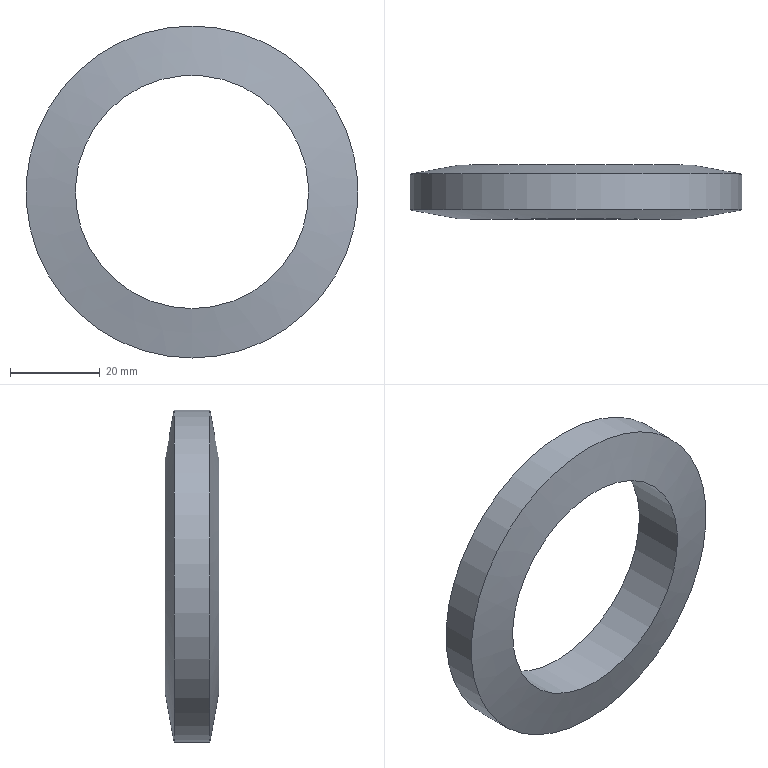Part | NX | features DATUM_CSYS 2, SKETCH 1, SWP104 1 | 1 solid | 4 faces | box 74 x 12 x 74 mm | volume 21518 mm3 | cone 2 | cylinder 2 | commonest cylinder face diameters 52 x1 74 x1
STEP:
#1=CARTESIAN_POINT('',(0.,-6.,-26.));
#2=VERTEX_POINT('',#1);
#3=CARTESIAN_POINT('',(0.,-6.,0.));
#4=DIRECTION('',(0.,-1.,0.));
#5=DIRECTION('',(0.,0.,-1.));
#6=AXIS2_PLACEMENT_3D('',#3,#4,#5);
#7=CIRCLE('',#6,26.);
#8=EDGE_CURVE('',#2,#2,#7,.T.);
#9=ORIENTED_EDGE('',*,*,#8,.F.);
#10=EDGE_LOOP('',(#9));
#11=FACE_BOUND('',#10,.T.);
#12=CARTESIAN_POINT('',(0.,-4.,-37.));
#13=VERTEX_POINT('',#12);
#14=CARTESIAN_POINT('',(0.,-4.,0.));
#15=DIRECTION('',(0.,-1.,0.));
#16=DIRECTION('',(0.,0.,-1.));
#17=AXIS2_PLACEMENT_3D('',#14,#15,#16);
#18=CIRCLE('',#17,37.);
#19=EDGE_CURVE('',#13,#13,#18,.T.);
#20=ORIENTED_EDGE('',*,*,#19,.T.);
#21=EDGE_LOOP('',(#20));
#22=FACE_BOUND('',#21,.T.);
#23=CARTESIAN_POINT('',(0.,-4.,0.));
#24=DIRECTION('',(0.,1.,0.));
#25=DIRECTION('',(0.,0.,1.));
#26=AXIS2_PLACEMENT_3D('',#23,#24,#25);
#27=CONICAL_SURFACE('',#26,37.,1.391);
#28=ADVANCED_FACE('',(#11,#22),#27,.T.);
#29=CARTESIAN_POINT('',(0.,6.,-26.));
#30=VERTEX_POINT('',#29);
#31=CARTESIAN_POINT('',(0.,6.,0.));
#32=DIRECTION('',(0.,-1.,0.));
#33=DIRECTION('',(0.,0.,-1.));
#34=AXIS2_PLACEMENT_3D('',#31,#32,#33);
#35=CIRCLE('',#34,26.);
#36=EDGE_CURVE('',#30,#30,#35,.T.);
#37=ORIENTED_EDGE('',*,*,#36,.F.);
#38=EDGE_LOOP('',(#37));
#39=FACE_BOUND('',#38,.T.);
#40=ORIENTED_EDGE('',*,*,#8,.T.);
#41=EDGE_LOOP('',(#40));
#42=FACE_BOUND('',#41,.T.);
#43=CARTESIAN_POINT('',(0.,0.,0.));
#44=DIRECTION('',(0.,-1.,0.));
#45=DIRECTION('',(0.,0.,-1.));
#46=AXIS2_PLACEMENT_3D('',#43,#44,#45);
#47=CYLINDRICAL_SURFACE('',#46,26.);
#48=ADVANCED_FACE('',(#39,#42),#47,.F.);
#49=CARTESIAN_POINT('',(0.,4.,-37.));
#50=VERTEX_POINT('',#49);
#51=CARTESIAN_POINT('',(0.,4.,0.));
#52=DIRECTION('',(0.,-1.,0.));
#53=DIRECTION('',(0.,0.,-1.));
#54=AXIS2_PLACEMENT_3D('',#51,#52,#53);
#55=CIRCLE('',#54,37.);
#56=EDGE_CURVE('',#50,#50,#55,.T.);
#57=ORIENTED_EDGE('',*,*,#56,.F.);
#58=EDGE_LOOP('',(#57));
#59=FACE_BOUND('',#58,.T.);
#60=ORIENTED_EDGE('',*,*,#36,.T.);
#61=EDGE_LOOP('',(#60));
#62=FACE_BOUND('',#61,.T.);
#63=CARTESIAN_POINT('',(0.,6.,0.));
#64=DIRECTION('',(0.,-1.,0.));
#65=DIRECTION('',(0.,0.,-1.));
#66=AXIS2_PLACEMENT_3D('',#63,#64,#65);
#67=CONICAL_SURFACE('',#66,26.,1.391);
#68=ADVANCED_FACE('',(#59,#62),#67,.T.);
#69=ORIENTED_EDGE('',*,*,#19,.F.);
#70=EDGE_LOOP('',(#69));
#71=FACE_BOUND('',#70,.T.);
#72=ORIENTED_EDGE('',*,*,#56,.T.);
#73=EDGE_LOOP('',(#72));
#74=FACE_BOUND('',#73,.T.);
#75=CARTESIAN_POINT('',(0.,0.,0.));
#76=DIRECTION('',(0.,-1.,0.));
#77=DIRECTION('',(0.,0.,-1.));
#78=AXIS2_PLACEMENT_3D('',#75,#76,#77);
#79=CYLINDRICAL_SURFACE('',#78,37.);
#80=ADVANCED_FACE('',(#71,#74),#79,.T.);
#81=CLOSED_SHELL('',(#28,#48,#68,#80));
#82=MANIFOLD_SOLID_BREP('',#81);
#83=(LENGTH_UNIT()NAMED_UNIT(*)SI_UNIT(.MILLI.,.METRE.));
#84=UNCERTAINTY_MEASURE_WITH_UNIT(LENGTH_MEASURE(0.00001),#83,'','');
#85=(NAMED_UNIT(*)PLANE_ANGLE_UNIT()SI_UNIT($,.RADIAN.));
#86=(NAMED_UNIT(*)SI_UNIT($,.STERADIAN.)SOLID_ANGLE_UNIT());
#87=(GEOMETRIC_REPRESENTATION_CONTEXT(3)GLOBAL_UNCERTAINTY_ASSIGNED_CONTEXT((#84))GLOBAL_UNIT_ASSIGNED_CONTEXT((#83,#85,#86))REPRESENTATION_CONTEXT('',''));
#88=ADVANCED_BREP_SHAPE_REPRESENTATION('',(#82),#87);